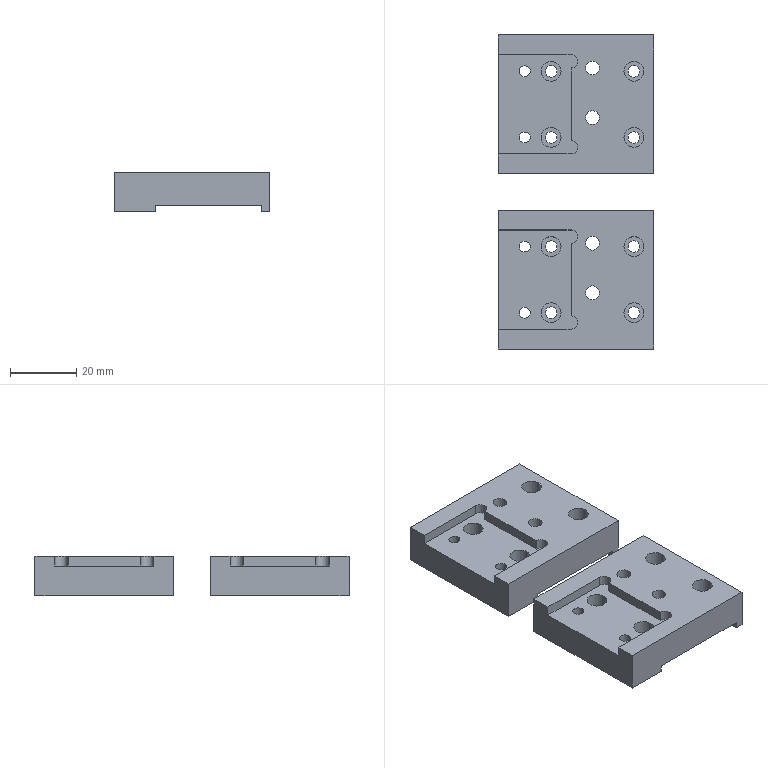NC program | NX | posted with a generic post | part box 47 x 95 x 12 mm
Whole program:
N10 G17 G21 G94 G90
(FLOOR_WALL_COPY_1 , TOOL : D80)
N12 T19 M6
N14 G54
N16 G17 G0 G90 X-90.5 Y0. S6500 M3
N18 G43 Z30. H19
N20 Z5.
N22 G94 G1 Z2. F1500.
N24 X-87.5
N26 X87.5
N28 X90.5
N30 Z5.
N32 G0 Z30.
N34 X-90.5
N36 Z4.
N38 G1 Z1.
N40 X-87.5
N42 X87.5
N44 X90.5
N46 Z4.
N48 G0 Z30.
N50 X-90.5
N52 Z3.
N54 G1 Z0.
N56 X-87.5
N58 X87.5
N60 X90.5
N62 Z3.
N64 G0 Z30.
N66 M5
(FLOOR_WALL_1_COPY , TOOL : D10)
N68 T15 M6
N70 G54
N72 G17 G0 G90 X-54. Y0.67 S9500 M3
N74 G43 Z30. H15
N76 Z0.55
N78 G94 G1 Z-0.95 F3000.
N80 X-48. Y4.134
N82 G3 X-47.5 Y5. R1.
N84 G1 Y15.9
N86 X-5.5
N88 Y-5.9
N90 X-47.5
N92 Y5.
N94 X-40.5
N96 Y8.9
N98 X-12.5
N100 Y1.1
N102 X-40.5
N104 Y5.
N106 G3 X-41. Y5.866 R1.
N108 G1 Z0.55
N110 G0 X-54. Y0.67 Z-0.4
N112 G1 Z-1.9
N114 X-48. Y4.134
N116 G3 X-47.5 Y5. R1.
N118 G1 Y15.9
N120 X-5.5
N122 Y-5.9
N124 X-47.5
N126 Y5.
N128 X-40.5
N130 Y8.9
N132 X-12.5
N134 Y1.1
N136 X-40.5
N138 Y5.
N140 G3 X-41. Y5.866 R1.
N142 G1 Z-0.4
N144 G0 Z3.
N146 X-1. Y0.67
N148 Z0.55
N150 G1 Z-0.95
N152 X5. Y4.134
N154 G3 X5.5 Y5. R1.
N156 G1 Y15.9
N158 X47.5
N160 Y-5.9
N162 X5.5
N164 Y5.
N166 X12.5
N168 Y8.9
N170 X40.5
N172 Y1.1
N174 X12.5
N176 Y5.
N178 G3 X12. Y5.866 R1.
N180 G1 Z0.55
N182 G0 X-1. Y0.67 Z-0.4
N184 G1 Z-1.9
N186 X5. Y4.134
N188 G3 X5.5 Y5. R1.
N190 G1 Y15.9
N192 X47.5
N194 Y-5.9
N196 X5.5
N198 Y5.
N200 X12.5
N202 Y8.9
N204 X40.5
N206 Y1.1
N208 X12.5
N210 Y5.
N212 G3 X12. Y5.866 R1.
N214 G1 Z-0.4
N216 G0 Z30.
N218 M5
(FLOOR_WALL_COPY_COPY , TOOL : D10JING)
N220 T14 M6
N222 G54
N224 G17 G0 G90 X-54. Y14.4 S9500 M3
N226 G43 Z30. H14
N228 Z-0.5
N230 G94 G1 Z-2. F1500.
N232 X-51.634 Y14.899
N234 G3 X-52.5 Y15.399 R1.
N236 G1 X-0.5
N238 Y11.239
N240 X-52.5
N242 Y7.079
N244 X-0.5
N246 Y2.92
N248 X-52.5
N250 Y-1.24
N252 X-0.5
N254 Y-5.4
N256 X-52.5
N258 G2 X-53.366 Y-4.9 R1.
N260 G1 X-54. Y-3.802
N262 Z-0.5
N264 G0 Y-4.302
N266 G1 Z-2.
N268 X-53.366 Y-5.4
N270 G3 X-52.5 Y-5.9 R1.
N272 G1 X-0.5
N274 G3 X-1. Y-5.034 R1.
N276 G1 X-2.964 Y-3.9
N278 Z-0.5
N280 G0 Y13.9
N282 G1 Z-2.
N284 X-1. Y15.034
N286 G3 X-0.5 Y15.9 R1.
N288 G1 X-52.5
N290 G3 X-53.366 Y15.4 R1.
N292 G1 X-54. Y14.302
N294 Z-0.5
N296 G0 Z1.1
N298 X-1. Y14.4
N300 Z-0.5
N302 G1 Z-2.
N304 X1.366 Y14.899
N306 G3 X0.5 Y15.399 R1.
N308 G1 X52.5
N310 Y11.239
N312 X0.5
N314 Y7.079
N316 X52.5
N318 Y2.92
N320 X0.5
N322 Y-1.24
N324 X52.5
N326 Y-5.4
N328 X0.5
N330 G2 X-0.366 Y-4.9 R1.
N332 G1 X-1. Y-3.802
N334 Z-0.5
N336 G0 Y-4.302
N338 G1 Z-2.
N340 X-0.366 Y-5.4
N342 G3 X0.5 Y-5.9 R1.
N344 G1 X52.5
N346 G3 X53.366 Y-5.4 R1.
N348 G1 X54. Y-4.302
N350 Z-0.5
N352 G0 Y14.302
N354 G1 Z-2.
N356 X53.366 Y15.4
N358 G3 X52.5 Y15.9 R1.
N360 G1 X0.5
N362 G3 X-0.366 Y15.4 R1.
N364 G1 X-1. Y14.302
N366 Z-0.5
N368 G0 Z30.
N370 M5
(PLANAR_MILL_COPY_COPY_COPY_COPY , TOOL : D6A45)
N372 T01 M6
N374 G54
N376 G17 G0 G90 X-27.366 Y24.9 S9500 M3
N378 G43 Z30. H1
N380 Z0.5
N382 G94 G1 Z-1. F1250.
N384 G3 X-26.5 Y24.4 R1.
N386 G1 X-5.5
N388 G2 X-4.6 Y23.5 R0.9
N390 G1 Y21.
N392 G2 X-5.5 Y20.1 R0.9
N394 G1 X-47.5
N396 G2 X-48.4 Y21. R0.9
N398 G1 Y23.5
N400 G2 X-47.5 Y24.4 R0.9
N402 G1 X-26.5
N404 G3 X-25.634 Y24.9 R1.
N406 G1 Z0.5
N408 G0 Z30.
N410 X-36.933 Y-16.
N412 Z0.5
N414 G1 Z-1.
N416 G3 X-36.5 Y-16.25 R0.5
N418 X-35.75 Y-15.5 R0.75
N420 X-36.5 Y-16.25 R-0.75
N422 X-36.067 Y-16. R0.5
N424 G1 Z0.5
N426 G0 Z30.
N428 X-25.634 Y-24.9
N430 Z0.5
N432 G1 Z-1.
N434 G3 X-26.5 Y-24.4 R1.
N436 G1 X-47.5
N438 G2 X-48.4 Y-23.5 R0.9
N440 G1 Y-11.
N442 G2 X-47.5 Y-10.1 R0.9
N444 G1 X-5.5
N446 G2 X-4.6 Y-11. R0.9
N448 G1 Y-23.5
N450 G2 X-5.5 Y-24.4 R0.9
N452 G1 X-26.5
N454 G3 X-27.366 Y-24.9 R1.
N456 G1 Z0.5
N458 G0 Z30.
N460 X-16.933 Y-16.
N462 Z0.5
N464 G1 Z-1.
N466 G3 X-16.5 Y-16.25 R0.5
N468 X-15.75 Y-15.5 R0.75
N470 X-16.5 Y-16.25 R-0.75
N472 X-16.067 Y-16. R0.5
N474 G1 Z0.5
N476 G0 Z30.
N478 X16.067
N480 Z0.5
N482 G1 Z-1.
N484 G3 X16.5 Y-16.25 R0.5
N486 X17.25 Y-15.5 R0.75
N488 X16.5 Y-16.25 R-0.75
N490 X16.933 Y-16. R0.5
N492 G1 Z0.5
N494 G0 Z30.
N496 X27.366 Y-24.9
N498 Z0.5
N500 G1 Z-1.
N502 G3 X26.5 Y-24.4 R1.
N504 G1 X5.5
N506 G2 X4.6 Y-23.5 R0.9
N508 G1 Y-11.
N510 G2 X5.5 Y-10.1 R0.9
N512 G1 X47.5
N514 G2 X48.4 Y-11. R0.9
N516 G1 Y-23.5
N518 G2 X47.5 Y-24.4 R0.9
N520 G1 X26.5
N522 G3 X25.634 Y-24.9 R1.
N524 G1 Z0.5
N526 G0 Z30.
N528 X36.067 Y-16.
N530 Z0.5
N532 G1 Z-1.
N534 G3 X36.5 Y-16.25 R0.5
N536 X37.25 Y-15.5 R0.75
N538 X36.5 Y-16.25 R-0.75
N540 X36.933 Y-16. R0.5
N542 G1 Z0.5
N544 G0 Z30.
N546 X25.634 Y24.9
N548 Z0.5
N550 G1 Z-1.
N552 G3 X26.5 Y24.4 R1.
N554 G1 X47.5
N556 G2 X48.4 Y23.5 R0.9
N558 G1 Y21.
N560 G2 X47.5 Y20.1 R0.9
N562 G1 X5.5
N564 G2 X4.6 Y21. R0.9
N566 G1 Y23.5
N568 G2 X5.5 Y24.4 R0.9
N570 G1 X26.5
N572 G3 X27.366 Y24.9 R1.
N574 G1 Z0.5
N576 G0 Z30.
N578 M5
(刀补_COPY , TOOL : D4)
N580 T11 M6
N582 G54
N584 G17 G0 G90 X-50.631 Y-7.356 S9500 M3
N586 G43 Z30. H11
N588 Z-0.5
N590 G94 G1 Z-2. F1500.
N592 G41 X-50.597 Y-7.45 D11
N594 X-49.846 Y-8.75
N596 G3 X-49.5 Y-8.95 R0.4
N598 G1 X-3.5
N600 G3 X-3.154 Y-8.75 R0.4
N602 G1 X-2.403 Y-7.45
N604 G40
N606 X-2.369 Y-7.356
N608 Z-0.5
N610 G0 Y17.356
N612 G1 Z-2.
N614 G41 X-2.403 Y17.45
N616 X-3.154 Y18.75
N618 G3 X-3.5 Y18.95 R0.4
N620 G1 X-49.5
N622 G3 X-49.846 Y18.75 R0.4
N624 G1 X-50.597 Y17.45
N626 G40
N628 X-50.631 Y17.356
N630 Z-0.5
N632 G0 Z1.1
N634 X2.369 Y-7.356
N636 Z-0.5
N638 G1 Z-2.
N640 G41 X2.403 Y-7.45
N642 X3.154 Y-8.75
N644 G3 X3.5 Y-8.95 R0.4
N646 G1 X49.5
N648 G3 X49.846 Y-8.75 R0.4
N650 G1 X50.597 Y-7.45
N652 G40
N654 X50.631 Y-7.356
N656 Z-0.5
N658 G0 Y17.356
N660 G1 Z-2.
N662 G41 X50.597 Y17.45
N664 X49.846 Y18.75
N666 G3 X49.5 Y18.95 R0.4
N668 G1 X3.5
N670 G3 X3.154 Y18.75 R0.4
N672 G1 X2.403 Y17.45
N674 G40
N676 X2.369 Y17.356
N678 Z-0.5
N680 G0 Z30.
N682 M5
N684 M2